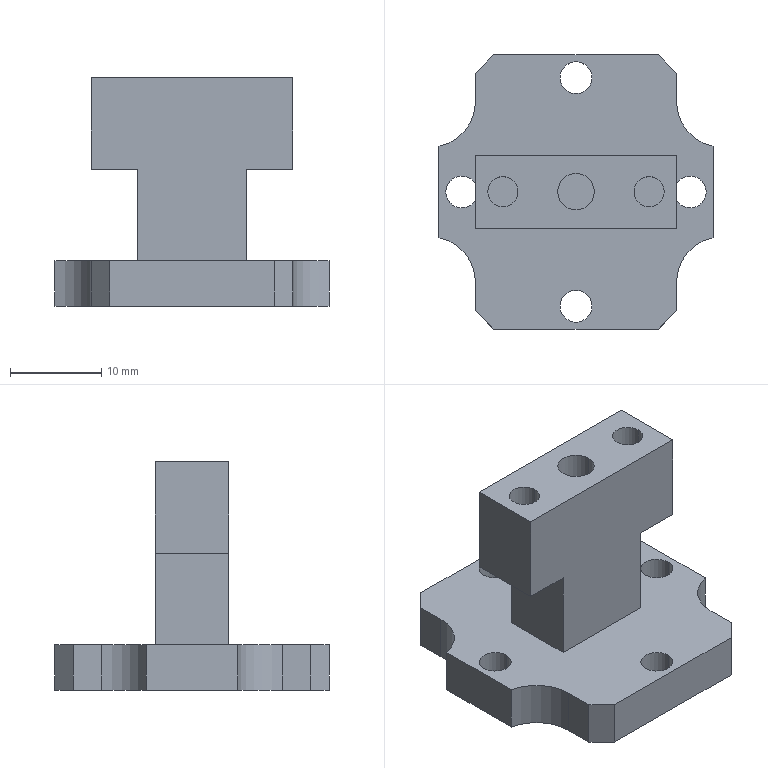Part | STEP file | 08-20 rotary support seat | 1 solid | 42 faces | box 30 x 30 x 25 mm | volume 6052 mm3 | plane 24 | cylinder 18 | commonest cylinder face diameters 3.5 x8 3.3 x4 10 x4 4 x2
STEP:
#1=CARTESIAN_POINT('',(10.75,0.,0.));
#2=VERTEX_POINT('',#1);
#3=CARTESIAN_POINT('',(14.25,0.,0.));
#4=VERTEX_POINT('',#3);
#5=CARTESIAN_POINT('',(12.5,0.,0.));
#6=DIRECTION('',(0.,0.,1.));
#7=DIRECTION('',(1.,0.,0.));
#8=AXIS2_PLACEMENT_3D('',#5,#6,#7);
#9=CIRCLE('',#8,1.75);
#10=EDGE_CURVE('',#2,#4,#9,.T.);
#11=ORIENTED_EDGE('',*,*,#10,.F.);
#12=CARTESIAN_POINT('',(10.75,0.,5.));
#13=VERTEX_POINT('',#12);
#14=CARTESIAN_POINT('',(10.75,0.,-5.));
#15=DIRECTION('',(0.,0.,1.));
#16=VECTOR('',#15,1000.);
#17=LINE('',#14,#16);
#18=EDGE_CURVE('',#2,#13,#17,.T.);
#19=ORIENTED_EDGE('',*,*,#18,.T.);
#20=CARTESIAN_POINT('',(14.25,0.,5.));
#21=VERTEX_POINT('',#20);
#22=CARTESIAN_POINT('',(12.5,0.,5.));
#23=DIRECTION('',(0.,0.,1.));
#24=DIRECTION('',(0.,1.,0.));
#25=AXIS2_PLACEMENT_3D('',#22,#23,#24);
#26=CIRCLE('',#25,1.75);
#27=EDGE_CURVE('',#13,#21,#26,.T.);
#28=ORIENTED_EDGE('',*,*,#27,.T.);
#29=CARTESIAN_POINT('',(14.25,0.,-5.));
#30=DIRECTION('',(0.,0.,1.));
#31=VECTOR('',#30,1000.);
#32=LINE('',#29,#31);
#33=EDGE_CURVE('',#4,#21,#32,.T.);
#34=ORIENTED_EDGE('',*,*,#33,.F.);
#35=EDGE_LOOP('',(#11,#19,#28,#34));
#36=FACE_OUTER_BOUND('',#35,.T.);
#37=CARTESIAN_POINT('',(12.5,0.,-5.));
#38=DIRECTION('',(0.,0.,1.));
#39=DIRECTION('',(1.,0.,0.));
#40=AXIS2_PLACEMENT_3D('',#37,#38,#39);
#41=CYLINDRICAL_SURFACE('',#40,1.75);
#42=ADVANCED_FACE('',(#36),#41,.F.);
#43=CARTESIAN_POINT('',(-14.25,0.,0.));
#44=VERTEX_POINT('',#43);
#45=CARTESIAN_POINT('',(-10.75,0.,0.));
#46=VERTEX_POINT('',#45);
#47=CARTESIAN_POINT('',(-12.5,0.,0.));
#48=DIRECTION('',(0.,0.,1.));
#49=DIRECTION('',(1.,0.,0.));
#50=AXIS2_PLACEMENT_3D('',#47,#48,#49);
#51=CIRCLE('',#50,1.75);
#52=EDGE_CURVE('',#44,#46,#51,.T.);
#53=ORIENTED_EDGE('',*,*,#52,.F.);
#54=CARTESIAN_POINT('',(-14.25,0.,5.));
#55=VERTEX_POINT('',#54);
#56=CARTESIAN_POINT('',(-14.25,0.,-5.));
#57=DIRECTION('',(0.,0.,1.));
#58=VECTOR('',#57,1000.);
#59=LINE('',#56,#58);
#60=EDGE_CURVE('',#44,#55,#59,.T.);
#61=ORIENTED_EDGE('',*,*,#60,.T.);
#62=CARTESIAN_POINT('',(-10.75,0.,5.));
#63=VERTEX_POINT('',#62);
#64=CARTESIAN_POINT('',(-12.5,0.,5.));
#65=DIRECTION('',(0.,0.,1.));
#66=DIRECTION('',(0.,1.,0.));
#67=AXIS2_PLACEMENT_3D('',#64,#65,#66);
#68=CIRCLE('',#67,1.75);
#69=EDGE_CURVE('',#55,#63,#68,.T.);
#70=ORIENTED_EDGE('',*,*,#69,.T.);
#71=CARTESIAN_POINT('',(-10.75,0.,-5.));
#72=DIRECTION('',(0.,0.,1.));
#73=VECTOR('',#72,1000.);
#74=LINE('',#71,#73);
#75=EDGE_CURVE('',#46,#63,#74,.T.);
#76=ORIENTED_EDGE('',*,*,#75,.F.);
#77=EDGE_LOOP('',(#53,#61,#70,#76));
#78=FACE_OUTER_BOUND('',#77,.T.);
#79=CARTESIAN_POINT('',(-12.5,0.,-5.));
#80=DIRECTION('',(0.,0.,1.));
#81=DIRECTION('',(1.,0.,0.));
#82=AXIS2_PLACEMENT_3D('',#79,#80,#81);
#83=CYLINDRICAL_SURFACE('',#82,1.75);
#84=ADVANCED_FACE('',(#78),#83,.F.);
#85=CARTESIAN_POINT('',(-1.75,-12.5,0.));
#86=VERTEX_POINT('',#85);
#87=CARTESIAN_POINT('',(1.75,-12.5,0.));
#88=VERTEX_POINT('',#87);
#89=CARTESIAN_POINT('',(0.,-12.5,0.));
#90=DIRECTION('',(0.,0.,1.));
#91=DIRECTION('',(1.,0.,0.));
#92=AXIS2_PLACEMENT_3D('',#89,#90,#91);
#93=CIRCLE('',#92,1.75);
#94=EDGE_CURVE('',#86,#88,#93,.T.);
#95=ORIENTED_EDGE('',*,*,#94,.F.);
#96=CARTESIAN_POINT('',(-1.75,-12.5,5.));
#97=VERTEX_POINT('',#96);
#98=CARTESIAN_POINT('',(-1.75,-12.5,-5.));
#99=DIRECTION('',(0.,0.,1.));
#100=VECTOR('',#99,1000.);
#101=LINE('',#98,#100);
#102=EDGE_CURVE('',#86,#97,#101,.T.);
#103=ORIENTED_EDGE('',*,*,#102,.T.);
#104=CARTESIAN_POINT('',(1.75,-12.5,5.));
#105=VERTEX_POINT('',#104);
#106=CARTESIAN_POINT('',(0.,-12.5,5.));
#107=DIRECTION('',(0.,0.,1.));
#108=DIRECTION('',(1.,0.,0.));
#109=AXIS2_PLACEMENT_3D('',#106,#107,#108);
#110=CIRCLE('',#109,1.75);
#111=EDGE_CURVE('',#97,#105,#110,.T.);
#112=ORIENTED_EDGE('',*,*,#111,.T.);
#113=CARTESIAN_POINT('',(1.75,-12.5,-5.));
#114=DIRECTION('',(0.,0.,1.));
#115=VECTOR('',#114,1000.);
#116=LINE('',#113,#115);
#117=EDGE_CURVE('',#88,#105,#116,.T.);
#118=ORIENTED_EDGE('',*,*,#117,.F.);
#119=EDGE_LOOP('',(#95,#103,#112,#118));
#120=FACE_OUTER_BOUND('',#119,.T.);
#121=CARTESIAN_POINT('',(0.,-12.5,-5.));
#122=DIRECTION('',(0.,0.,1.));
#123=DIRECTION('',(1.,0.,0.));
#124=AXIS2_PLACEMENT_3D('',#121,#122,#123);
#125=CYLINDRICAL_SURFACE('',#124,1.75);
#126=ADVANCED_FACE('',(#120),#125,.F.);
#127=CARTESIAN_POINT('',(-1.75,12.5,0.));
#128=VERTEX_POINT('',#127);
#129=CARTESIAN_POINT('',(1.75,12.5,0.));
#130=VERTEX_POINT('',#129);
#131=CARTESIAN_POINT('',(0.,12.5,0.));
#132=DIRECTION('',(0.,0.,1.));
#133=DIRECTION('',(1.,0.,0.));
#134=AXIS2_PLACEMENT_3D('',#131,#132,#133);
#135=CIRCLE('',#134,1.75);
#136=EDGE_CURVE('',#128,#130,#135,.T.);
#137=ORIENTED_EDGE('',*,*,#136,.F.);
#138=CARTESIAN_POINT('',(-1.75,12.5,5.));
#139=VERTEX_POINT('',#138);
#140=CARTESIAN_POINT('',(-1.75,12.5,-5.));
#141=DIRECTION('',(0.,0.,1.));
#142=VECTOR('',#141,1000.);
#143=LINE('',#140,#142);
#144=EDGE_CURVE('',#128,#139,#143,.T.);
#145=ORIENTED_EDGE('',*,*,#144,.T.);
#146=CARTESIAN_POINT('',(1.75,12.5,5.));
#147=VERTEX_POINT('',#146);
#148=CARTESIAN_POINT('',(0.,12.5,5.));
#149=DIRECTION('',(0.,0.,1.));
#150=DIRECTION('',(1.,0.,0.));
#151=AXIS2_PLACEMENT_3D('',#148,#149,#150);
#152=CIRCLE('',#151,1.75);
#153=EDGE_CURVE('',#139,#147,#152,.T.);
#154=ORIENTED_EDGE('',*,*,#153,.T.);
#155=CARTESIAN_POINT('',(1.75,12.5,-5.));
#156=DIRECTION('',(0.,0.,1.));
#157=VECTOR('',#156,1000.);
#158=LINE('',#155,#157);
#159=EDGE_CURVE('',#130,#147,#158,.T.);
#160=ORIENTED_EDGE('',*,*,#159,.F.);
#161=EDGE_LOOP('',(#137,#145,#154,#160));
#162=FACE_OUTER_BOUND('',#161,.T.);
#163=CARTESIAN_POINT('',(0.,12.5,-5.));
#164=DIRECTION('',(0.,0.,1.));
#165=DIRECTION('',(1.,0.,0.));
#166=AXIS2_PLACEMENT_3D('',#163,#164,#165);
#167=CYLINDRICAL_SURFACE('',#166,1.75);
#168=ADVANCED_FACE('',(#162),#167,.F.);
#169=CARTESIAN_POINT('',(-6.35,0.,15.));
#170=VERTEX_POINT('',#169);
#171=CARTESIAN_POINT('',(-9.65,0.,15.));
#172=VERTEX_POINT('',#171);
#173=CARTESIAN_POINT('',(-8.,0.,15.));
#174=DIRECTION('',(0.,0.,-1.));
#175=DIRECTION('',(1.,0.,0.));
#176=AXIS2_PLACEMENT_3D('',#173,#174,#175);
#177=CIRCLE('',#176,1.65);
#178=EDGE_CURVE('',#170,#172,#177,.T.);
#179=ORIENTED_EDGE('',*,*,#178,.T.);
#180=CARTESIAN_POINT('',(-9.65,0.,25.));
#181=VERTEX_POINT('',#180);
#182=CARTESIAN_POINT('',(-9.65,0.,25.));
#183=DIRECTION('',(0.,0.,1.));
#184=VECTOR('',#183,1000.);
#185=LINE('',#182,#184);
#186=EDGE_CURVE('',#172,#181,#185,.T.);
#187=ORIENTED_EDGE('',*,*,#186,.T.);
#188=CARTESIAN_POINT('',(-6.35,0.,25.));
#189=VERTEX_POINT('',#188);
#190=CARTESIAN_POINT('',(-8.,0.,25.));
#191=DIRECTION('',(0.,0.,1.));
#192=DIRECTION('',(1.,0.,0.));
#193=AXIS2_PLACEMENT_3D('',#190,#191,#192);
#194=CIRCLE('',#193,1.65);
#195=EDGE_CURVE('',#181,#189,#194,.T.);
#196=ORIENTED_EDGE('',*,*,#195,.T.);
#197=CARTESIAN_POINT('',(-6.35,0.,25.));
#198=DIRECTION('',(0.,0.,1.));
#199=VECTOR('',#198,1000.);
#200=LINE('',#197,#199);
#201=EDGE_CURVE('',#170,#189,#200,.T.);
#202=ORIENTED_EDGE('',*,*,#201,.F.);
#203=EDGE_LOOP('',(#179,#187,#196,#202));
#204=FACE_OUTER_BOUND('',#203,.T.);
#205=CARTESIAN_POINT('',(-8.,0.,25.));
#206=DIRECTION('',(0.,0.,1.));
#207=DIRECTION('',(1.,0.,0.));
#208=AXIS2_PLACEMENT_3D('',#205,#206,#207);
#209=CYLINDRICAL_SURFACE('',#208,1.65);
#210=ADVANCED_FACE('',(#204),#209,.F.);
#211=CARTESIAN_POINT('',(9.65,0.,15.));
#212=VERTEX_POINT('',#211);
#213=CARTESIAN_POINT('',(6.35,0.,15.));
#214=VERTEX_POINT('',#213);
#215=CARTESIAN_POINT('',(8.,0.,15.));
#216=DIRECTION('',(0.,0.,-1.));
#217=DIRECTION('',(1.,0.,0.));
#218=AXIS2_PLACEMENT_3D('',#215,#216,#217);
#219=CIRCLE('',#218,1.65);
#220=EDGE_CURVE('',#212,#214,#219,.T.);
#221=ORIENTED_EDGE('',*,*,#220,.T.);
#222=CARTESIAN_POINT('',(6.35,0.,25.));
#223=VERTEX_POINT('',#222);
#224=CARTESIAN_POINT('',(6.35,0.,25.));
#225=DIRECTION('',(0.,0.,1.));
#226=VECTOR('',#225,1000.);
#227=LINE('',#224,#226);
#228=EDGE_CURVE('',#214,#223,#227,.T.);
#229=ORIENTED_EDGE('',*,*,#228,.T.);
#230=CARTESIAN_POINT('',(9.65,0.,25.));
#231=VERTEX_POINT('',#230);
#232=CARTESIAN_POINT('',(8.,0.,25.));
#233=DIRECTION('',(0.,0.,1.));
#234=DIRECTION('',(1.,0.,0.));
#235=AXIS2_PLACEMENT_3D('',#232,#233,#234);
#236=CIRCLE('',#235,1.65);
#237=EDGE_CURVE('',#223,#231,#236,.T.);
#238=ORIENTED_EDGE('',*,*,#237,.T.);
#239=CARTESIAN_POINT('',(9.65,0.,25.));
#240=DIRECTION('',(0.,0.,1.));
#241=VECTOR('',#240,1000.);
#242=LINE('',#239,#241);
#243=EDGE_CURVE('',#212,#231,#242,.T.);
#244=ORIENTED_EDGE('',*,*,#243,.F.);
#245=EDGE_LOOP('',(#221,#229,#238,#244));
#246=FACE_OUTER_BOUND('',#245,.T.);
#247=CARTESIAN_POINT('',(8.,0.,25.));
#248=DIRECTION('',(0.,0.,1.));
#249=DIRECTION('',(1.,0.,0.));
#250=AXIS2_PLACEMENT_3D('',#247,#248,#249);
#251=CYLINDRICAL_SURFACE('',#250,1.65);
#252=ADVANCED_FACE('',(#246),#251,.F.);
#253=CARTESIAN_POINT('',(-2.,0.,20.));
#254=VERTEX_POINT('',#253);
#255=CARTESIAN_POINT('',(2.,0.,20.));
#256=VERTEX_POINT('',#255);
#257=CARTESIAN_POINT('',(0.,0.,20.));
#258=DIRECTION('',(0.,0.,1.));
#259=DIRECTION('',(1.,0.,0.));
#260=AXIS2_PLACEMENT_3D('',#257,#258,#259);
#261=CIRCLE('',#260,2.);
#262=EDGE_CURVE('',#254,#256,#261,.T.);
#263=ORIENTED_EDGE('',*,*,#262,.F.);
#264=CARTESIAN_POINT('',(-2.,0.,25.));
#265=VERTEX_POINT('',#264);
#266=CARTESIAN_POINT('',(-2.,0.,20.));
#267=DIRECTION('',(0.,0.,1.));
#268=VECTOR('',#267,1000.);
#269=LINE('',#266,#268);
#270=EDGE_CURVE('',#254,#265,#269,.T.);
#271=ORIENTED_EDGE('',*,*,#270,.T.);
#272=CARTESIAN_POINT('',(2.,0.,25.));
#273=VERTEX_POINT('',#272);
#274=CARTESIAN_POINT('',(0.,0.,25.));
#275=DIRECTION('',(0.,0.,1.));
#276=DIRECTION('',(1.,0.,0.));
#277=AXIS2_PLACEMENT_3D('',#274,#275,#276);
#278=CIRCLE('',#277,2.);
#279=EDGE_CURVE('',#265,#273,#278,.T.);
#280=ORIENTED_EDGE('',*,*,#279,.T.);
#281=CARTESIAN_POINT('',(2.,0.,20.));
#282=DIRECTION('',(0.,0.,1.));
#283=VECTOR('',#282,1000.);
#284=LINE('',#281,#283);
#285=EDGE_CURVE('',#256,#273,#284,.T.);
#286=ORIENTED_EDGE('',*,*,#285,.F.);
#287=EDGE_LOOP('',(#263,#271,#280,#286));
#288=FACE_OUTER_BOUND('',#287,.T.);
#289=CARTESIAN_POINT('',(0.,0.,20.));
#290=DIRECTION('',(0.,0.,1.));
#291=DIRECTION('',(1.,0.,0.));
#292=AXIS2_PLACEMENT_3D('',#289,#290,#291);
#293=CYLINDRICAL_SURFACE('',#292,2.);
#294=ADVANCED_FACE('',(#288),#293,.F.);
#295=CARTESIAN_POINT('',(11.,9.899,5.));
#296=VERTEX_POINT('',#295);
#297=CARTESIAN_POINT('',(11.,13.,5.));
#298=VERTEX_POINT('',#297);
#299=CARTESIAN_POINT('',(11.,15.,5.));
#300=DIRECTION('',(0.,1.,0.));
#301=VECTOR('',#300,1000.);
#302=LINE('',#299,#301);
#303=EDGE_CURVE('',#296,#298,#302,.T.);
#304=ORIENTED_EDGE('',*,*,#303,.F.);
#305=CARTESIAN_POINT('',(11.,9.899,0.));
#306=VERTEX_POINT('',#305);
#307=CARTESIAN_POINT('',(11.,9.899,5.));
#308=DIRECTION('',(0.,0.,-1.));
#309=VECTOR('',#308,1000.);
#310=LINE('',#307,#309);
#311=EDGE_CURVE('',#296,#306,#310,.T.);
#312=ORIENTED_EDGE('',*,*,#311,.T.);
#313=CARTESIAN_POINT('',(11.,13.,0.));
#314=VERTEX_POINT('',#313);
#315=CARTESIAN_POINT('',(11.,15.,0.));
#316=DIRECTION('',(0.,1.,0.));
#317=VECTOR('',#316,1000.);
#318=LINE('',#315,#317);
#319=EDGE_CURVE('',#306,#314,#318,.T.);
#320=ORIENTED_EDGE('',*,*,#319,.T.);
#321=CARTESIAN_POINT('',(11.,13.,5.));
#322=DIRECTION('',(0.,0.,1.));
#323=VECTOR('',#322,1000.);
#324=LINE('',#321,#323);
#325=EDGE_CURVE('',#314,#298,#324,.T.);
#326=ORIENTED_EDGE('',*,*,#325,.T.);
#327=EDGE_LOOP('',(#304,#312,#320,#326));
#328=FACE_OUTER_BOUND('',#327,.T.);
#329=CARTESIAN_POINT('',(11.,15.,5.));
#330=DIRECTION('',(-1.,0.,0.));
#331=DIRECTION('',(0.,-1.,0.));
#332=AXIS2_PLACEMENT_3D('',#329,#330,#331);
#333=PLANE('',#332);
#334=ADVANCED_FACE('',(#328),#333,.F.);
#335=CARTESIAN_POINT('',(11.,-4.,25.));
#336=VERTEX_POINT('',#335);
#337=CARTESIAN_POINT('',(11.,-4.,15.));
#338=VERTEX_POINT('',#337);
#339=CARTESIAN_POINT('',(11.,-4.,25.));
#340=DIRECTION('',(0.,0.,-1.));
#341=VECTOR('',#340,1000.);
#342=LINE('',#339,#341);
#343=EDGE_CURVE('',#336,#338,#342,.T.);
#344=ORIENTED_EDGE('',*,*,#343,.T.);
#345=CARTESIAN_POINT('',(11.,4.,15.));
#346=VERTEX_POINT('',#345);
#347=CARTESIAN_POINT('',(11.,-6.,15.));
#348=DIRECTION('',(0.,1.,0.));
#349=VECTOR('',#348,1000.);
#350=LINE('',#347,#349);
#351=EDGE_CURVE('',#338,#346,#350,.T.);
#352=ORIENTED_EDGE('',*,*,#351,.T.);
#353=CARTESIAN_POINT('',(11.,4.,25.));
#354=VERTEX_POINT('',#353);
#355=CARTESIAN_POINT('',(11.,4.,25.));
#356=DIRECTION('',(0.,0.,-1.));
#357=VECTOR('',#356,1000.);
#358=LINE('',#355,#357);
#359=EDGE_CURVE('',#354,#346,#358,.T.);
#360=ORIENTED_EDGE('',*,*,#359,.F.);
#361=CARTESIAN_POINT('',(11.,4.,25.));
#362=DIRECTION('',(0.,1.,0.));
#363=VECTOR('',#362,1000.);
#364=LINE('',#361,#363);
#365=EDGE_CURVE('',#336,#354,#364,.T.);
#366=ORIENTED_EDGE('',*,*,#365,.F.);
#367=EDGE_LOOP('',(#344,#352,#360,#366));
#368=FACE_OUTER_BOUND('',#367,.T.);
#369=CARTESIAN_POINT('',(11.,15.,5.));
#370=DIRECTION('',(-1.,0.,0.));
#371=DIRECTION('',(0.,-1.,0.));
#372=AXIS2_PLACEMENT_3D('',#369,#370,#371);
#373=PLANE('',#372);
#374=ADVANCED_FACE('',(#368),#373,.F.);
#375=CARTESIAN_POINT('',(-11.,13.,0.));
#376=VERTEX_POINT('',#375);
#377=CARTESIAN_POINT('',(-11.,9.899,0.));
#378=VERTEX_POINT('',#377);
#379=CARTESIAN_POINT('',(-11.,15.,0.));
#380=DIRECTION('',(0.,-1.,0.));
#381=VECTOR('',#380,1000.);
#382=LINE('',#379,#381);
#383=EDGE_CURVE('',#376,#378,#382,.T.);
#384=ORIENTED_EDGE('',*,*,#383,.T.);
#385=CARTESIAN_POINT('',(-11.,9.899,5.));
#386=VERTEX_POINT('',#385);
#387=CARTESIAN_POINT('',(-11.,9.899,5.));
#388=DIRECTION('',(0.,0.,1.));
#389=VECTOR('',#388,1000.);
#390=LINE('',#387,#389);
#391=EDGE_CURVE('',#378,#386,#390,.T.);
#392=ORIENTED_EDGE('',*,*,#391,.T.);
#393=CARTESIAN_POINT('',(-11.,13.,5.));
#394=VERTEX_POINT('',#393);
#395=CARTESIAN_POINT('',(-11.,15.,5.));
#396=DIRECTION('',(0.,-1.,0.));
#397=VECTOR('',#396,1000.);
#398=LINE('',#395,#397);
#399=EDGE_CURVE('',#394,#386,#398,.T.);
#400=ORIENTED_EDGE('',*,*,#399,.F.);
#401=CARTESIAN_POINT('',(-11.,13.,5.));
#402=DIRECTION('',(0.,0.,-1.));
#403=VECTOR('',#402,1000.);
#404=LINE('',#401,#403);
#405=EDGE_CURVE('',#394,#376,#404,.T.);
#406=ORIENTED_EDGE('',*,*,#405,.T.);
#407=EDGE_LOOP('',(#384,#392,#400,#406));
#408=FACE_OUTER_BOUND('',#407,.T.);
#409=CARTESIAN_POINT('',(-11.,15.,5.));
#410=DIRECTION('',(1.,0.,0.));
#411=DIRECTION('',(0.,1.,0.));
#412=AXIS2_PLACEMENT_3D('',#409,#410,#411);
#413=PLANE('',#412);
#414=ADVANCED_FACE('',(#408),#413,.F.);
#415=CARTESIAN_POINT('',(-11.,4.,25.));
#416=VERTEX_POINT('',#415);
#417=CARTESIAN_POINT('',(-11.,4.,15.));
#418=VERTEX_POINT('',#417);
#419=CARTESIAN_POINT('',(-11.,4.,25.));
#420=DIRECTION('',(0.,0.,-1.));
#421=VECTOR('',#420,1000.);
#422=LINE('',#419,#421);
#423=EDGE_CURVE('',#416,#418,#422,.T.);
#424=ORIENTED_EDGE('',*,*,#423,.T.);
#425=CARTESIAN_POINT('',(-11.,-4.,15.));
#426=VERTEX_POINT('',#425);
#427=CARTESIAN_POINT('',(-11.,-6.,15.));
#428=DIRECTION('',(0.,1.,0.));
#429=VECTOR('',#428,1000.);
#430=LINE('',#427,#429);
#431=EDGE_CURVE('',#426,#418,#430,.T.);
#432=ORIENTED_EDGE('',*,*,#431,.F.);
#433=CARTESIAN_POINT('',(-11.,-4.,25.));
#434=VERTEX_POINT('',#433);
#435=CARTESIAN_POINT('',(-11.,-4.,25.));
#436=DIRECTION('',(0.,0.,-1.));
#437=VECTOR('',#436,1000.);
#438=LINE('',#435,#437);
#439=EDGE_CURVE('',#434,#426,#438,.T.);
#440=ORIENTED_EDGE('',*,*,#439,.F.);
#441=CARTESIAN_POINT('',(-11.,4.,25.));
#442=DIRECTION('',(0.,-1.,0.));
#443=VECTOR('',#442,1000.);
#444=LINE('',#441,#443);
#445=EDGE_CURVE('',#416,#434,#444,.T.);
#446=ORIENTED_EDGE('',*,*,#445,.F.);
#447=EDGE_LOOP('',(#424,#432,#440,#446));
#448=FACE_OUTER_BOUND('',#447,.T.);
#449=CARTESIAN_POINT('',(-11.,15.,5.));
#450=DIRECTION('',(1.,0.,0.));
#451=DIRECTION('',(0.,1.,0.));
#452=AXIS2_PLACEMENT_3D('',#449,#450,#451);
#453=PLANE('',#452);
#454=ADVANCED_FACE('',(#448),#453,.F.);
#455=CARTESIAN_POINT('',(11.,-13.,0.));
#456=VERTEX_POINT('',#455);
#457=CARTESIAN_POINT('',(11.,-9.899,0.));
#458=VERTEX_POINT('',#457);
#459=CARTESIAN_POINT('',(11.,15.,0.));
#460=DIRECTION('',(0.,1.,0.));
#461=VECTOR('',#460,1000.);
#462=LINE('',#459,#461);
#463=EDGE_CURVE('',#456,#458,#462,.T.);
#464=ORIENTED_EDGE('',*,*,#463,.T.);
#465=CARTESIAN_POINT('',(11.,-9.899,5.));
#466=VERTEX_POINT('',#465);
#467=CARTESIAN_POINT('',(11.,-9.899,5.));
#468=DIRECTION('',(0.,0.,1.));
#469=VECTOR('',#468,1000.);
#470=LINE('',#467,#469);
#471=EDGE_CURVE('',#458,#466,#470,.T.);
#472=ORIENTED_EDGE('',*,*,#471,.T.);
#473=CARTESIAN_POINT('',(11.,-13.,5.));
#474=VERTEX_POINT('',#473);
#475=CARTESIAN_POINT('',(11.,15.,5.));
#476=DIRECTION('',(0.,1.,0.));
#477=VECTOR('',#476,1000.);
#478=LINE('',#475,#477);
#479=EDGE_CURVE('',#474,#466,#478,.T.);
#480=ORIENTED_EDGE('',*,*,#479,.F.);
#481=CARTESIAN_POINT('',(11.,-13.,5.));
#482=DIRECTION('',(0.,0.,-1.));
#483=VECTOR('',#482,1000.);
#484=LINE('',#481,#483);
#485=EDGE_CURVE('',#474,#456,#484,.T.);
#486=ORIENTED_EDGE('',*,*,#485,.T.);
#487=EDGE_LOOP('',(#464,#472,#480,#486));
#488=FACE_OUTER_BOUND('',#487,.T.);
#489=CARTESIAN_POINT('',(11.,15.,5.));
#490=DIRECTION('',(-1.,0.,0.));
#491=DIRECTION('',(0.,-1.,0.));
#492=AXIS2_PLACEMENT_3D('',#489,#490,#491);
#493=PLANE('',#492);
#494=ADVANCED_FACE('',(#488),#493,.F.);
#495=CARTESIAN_POINT('',(9.,15.,5.));
#496=VERTEX_POINT('',#495);
#497=CARTESIAN_POINT('',(-9.,15.,5.));
#498=VERTEX_POINT('',#497);
#499=CARTESIAN_POINT('',(-11.,15.,5.));
#500=DIRECTION('',(-1.,0.,0.));
#501=VECTOR('',#500,1000.);
#502=LINE('',#499,#501);
#503=EDGE_CURVE('',#496,#498,#502,.T.);
#504=ORIENTED_EDGE('',*,*,#503,.F.);
#505=CARTESIAN_POINT('',(9.,15.,0.));
#506=VERTEX_POINT('',#505);
#507=CARTESIAN_POINT('',(9.,15.,5.));
#508=DIRECTION('',(0.,0.,-1.));
#509=VECTOR('',#508,1000.);
#510=LINE('',#507,#509);
#511=EDGE_CURVE('',#496,#506,#510,.T.);
#512=ORIENTED_EDGE('',*,*,#511,.T.);
#513=CARTESIAN_POINT('',(-9.,15.,0.));
#514=VERTEX_POINT('',#513);
#515=CARTESIAN_POINT('',(-11.,15.,0.));
#516=DIRECTION('',(-1.,0.,0.));
#517=VECTOR('',#516,1000.);
#518=LINE('',#515,#517);
#519=EDGE_CURVE('',#506,#514,#518,.T.);
#520=ORIENTED_EDGE('',*,*,#519,.T.);
#521=CARTESIAN_POINT('',(-9.,15.,5.));
#522=DIRECTION('',(0.,0.,1.));
#523=VECTOR('',#522,1000.);
#524=LINE('',#521,#523);
#525=EDGE_CURVE('',#514,#498,#524,.T.);
#526=ORIENTED_EDGE('',*,*,#525,.T.);
#527=EDGE_LOOP('',(#504,#512,#520,#526));
#528=FACE_OUTER_BOUND('',#527,.T.);
#529=CARTESIAN_POINT('',(-11.,15.,5.));
#530=DIRECTION('',(0.,-1.,0.));
#531=DIRECTION('',(0.,0.,-1.));
#532=AXIS2_PLACEMENT_3D('',#529,#530,#531);
#533=PLANE('',#532);
#534=ADVANCED_FACE('',(#528),#533,.F.);
#535=CARTESIAN_POINT('',(-11.,-9.899,5.));
#536=VERTEX_POINT('',#535);
#537=CARTESIAN_POINT('',(-11.,-13.,5.));
#538=VERTEX_POINT('',#537);
#539=CARTESIAN_POINT('',(-11.,15.,5.));
#540=DIRECTION('',(0.,-1.,0.));
#541=VECTOR('',#540,1000.);
#542=LINE('',#539,#541);
#543=EDGE_CURVE('',#536,#538,#542,.T.);
#544=ORIENTED_EDGE('',*,*,#543,.F.);
#545=CARTESIAN_POINT('',(-11.,-9.899,0.));
#546=VERTEX_POINT('',#545);
#547=CARTESIAN_POINT('',(-11.,-9.899,5.));
#548=DIRECTION('',(0.,0.,-1.));
#549=VECTOR('',#548,1000.);
#550=LINE('',#547,#549);
#551=EDGE_CURVE('',#536,#546,#550,.T.);
#552=ORIENTED_EDGE('',*,*,#551,.T.);
#553=CARTESIAN_POINT('',(-11.,-13.,0.));
#554=VERTEX_POINT('',#553);
#555=CARTESIAN_POINT('',(-11.,15.,0.));
#556=DIRECTION('',(0.,-1.,0.));
#557=VECTOR('',#556,1000.);
#558=LINE('',#555,#557);
#559=EDGE_CURVE('',#546,#554,#558,.T.);
#560=ORIENTED_EDGE('',*,*,#559,.T.);
#561=CARTESIAN_POINT('',(-11.,-13.,5.));
#562=DIRECTION('',(0.,0.,1.));
#563=VECTOR('',#562,1000.);
#564=LINE('',#561,#563);
#565=EDGE_CURVE('',#554,#538,#564,.T.);
#566=ORIENTED_EDGE('',*,*,#565,.T.);
#567=EDGE_LOOP('',(#544,#552,#560,#566));
#568=FACE_OUTER_BOUND('',#567,.T.);
#569=CARTESIAN_POINT('',(-11.,15.,5.));
#570=DIRECTION('',(1.,0.,0.));
#571=DIRECTION('',(0.,1.,0.));
#572=AXIS2_PLACEMENT_3D('',#569,#570,#571);
#573=PLANE('',#572);
#574=ADVANCED_FACE('',(#568),#573,.F.);
#575=CARTESIAN_POINT('',(-9.,-15.,5.));
#576=VERTEX_POINT('',#575);
#577=CARTESIAN_POINT('',(9.,-15.,5.));
#578=VERTEX_POINT('',#577);
#579=CARTESIAN_POINT('',(-11.,-15.,5.));
#580=DIRECTION('',(1.,0.,0.));
#581=VECTOR('',#580,1000.);
#582=LINE('',#579,#581);
#583=EDGE_CURVE('',#576,#578,#582,.T.);
#584=ORIENTED_EDGE('',*,*,#583,.F.);
#585=CARTESIAN_POINT('',(-9.,-15.,0.));
#586=VERTEX_POINT('',#585);
#587=CARTESIAN_POINT('',(-9.,-15.,5.));
#588=DIRECTION('',(0.,0.,-1.));
#589=VECTOR('',#588,1000.);
#590=LINE('',#587,#589);
#591=EDGE_CURVE('',#576,#586,#590,.T.);
#592=ORIENTED_EDGE('',*,*,#591,.T.);
#593=CARTESIAN_POINT('',(9.,-15.,0.));
#594=VERTEX_POINT('',#593);
#595=CARTESIAN_POINT('',(-11.,-15.,0.));
#596=DIRECTION('',(1.,0.,0.));
#597=VECTOR('',#596,1000.);
#598=LINE('',#595,#597);
#599=EDGE_CURVE('',#586,#594,#598,.T.);
#600=ORIENTED_EDGE('',*,*,#599,.T.);
#601=CARTESIAN_POINT('',(9.,-15.,5.));
#602=DIRECTION('',(0.,0.,1.));
#603=VECTOR('',#602,1000.);
#604=LINE('',#601,#603);
#605=EDGE_CURVE('',#594,#578,#604,.T.);
#606=ORIENTED_EDGE('',*,*,#605,.T.);
#607=EDGE_LOOP('',(#584,#592,#600,#606));
#608=FACE_OUTER_BOUND('',#607,.T.);
#609=CARTESIAN_POINT('',(-11.,-15.,5.));
#610=DIRECTION('',(0.,1.,0.));
#611=DIRECTION('',(0.,0.,1.));
#612=AXIS2_PLACEMENT_3D('',#609,#610,#611);
#613=PLANE('',#612);
#614=ADVANCED_FACE('',(#608),#613,.F.);
#615=CARTESIAN_POINT('',(12.5,0.,5.));
#616=DIRECTION('',(0.,0.,1.));
#617=DIRECTION('',(0.,1.,0.));
#618=AXIS2_PLACEMENT_3D('',#615,#616,#617);
#619=CIRCLE('',#618,1.75);
#620=EDGE_CURVE('',#21,#13,#619,.T.);
#621=ORIENTED_EDGE('',*,*,#620,.F.);
#622=ORIENTED_EDGE('',*,*,#27,.F.);
#623=EDGE_LOOP('',(#621,#622));
#624=FACE_BOUND('',#623,.T.);
#625=CARTESIAN_POINT('',(6.,-4.,5.));
#626=VERTEX_POINT('',#625);
#627=CARTESIAN_POINT('',(6.,4.,5.));
#628=VERTEX_POINT('',#627);
#629=CARTESIAN_POINT('',(6.,-6.,5.));
#630=DIRECTION('',(0.,1.,0.));
#631=VECTOR('',#630,1000.);
#632=LINE('',#629,#631);
#633=EDGE_CURVE('',#626,#628,#632,.T.);
#634=ORIENTED_EDGE('',*,*,#633,.F.);
#635=CARTESIAN_POINT('',(-6.,-4.,5.));
#636=VERTEX_POINT('',#635);
#637=CARTESIAN_POINT('',(-11.,-4.,5.));
#638=DIRECTION('',(1.,0.,0.));
#639=VECTOR('',#638,1000.);
#640=LINE('',#637,#639);
#641=EDGE_CURVE('',#636,#626,#640,.T.);
#642=ORIENTED_EDGE('',*,*,#641,.F.);
#643=CARTESIAN_POINT('',(-6.,4.,5.));
#644=VERTEX_POINT('',#643);
#645=CARTESIAN_POINT('',(-6.,-6.,5.));
#646=DIRECTION('',(0.,1.,0.));
#647=VECTOR('',#646,1000.);
#648=LINE('',#645,#647);
#649=EDGE_CURVE('',#636,#644,#648,.T.);
#650=ORIENTED_EDGE('',*,*,#649,.T.);
#651=CARTESIAN_POINT('',(-11.,4.,5.));
#652=DIRECTION('',(-1.,0.,0.));
#653=VECTOR('',#652,1000.);
#654=LINE('',#651,#653);
#655=EDGE_CURVE('',#628,#644,#654,.T.);
#656=ORIENTED_EDGE('',*,*,#655,.F.);
#657=EDGE_LOOP('',(#634,#642,#650,#656));
#658=FACE_BOUND('',#657,.T.);
#659=CARTESIAN_POINT('',(-12.5,0.,5.));
#660=DIRECTION('',(0.,0.,1.));
#661=DIRECTION('',(0.,1.,0.));
#662=AXIS2_PLACEMENT_3D('',#659,#660,#661);
#663=CIRCLE('',#662,1.75);
#664=EDGE_CURVE('',#63,#55,#663,.T.);
#665=ORIENTED_EDGE('',*,*,#664,.F.);
#666=ORIENTED_EDGE('',*,*,#69,.F.);
#667=EDGE_LOOP('',(#665,#666));
#668=FACE_BOUND('',#667,.T.);
#669=CARTESIAN_POINT('',(15.,-5.,5.));
#670=VERTEX_POINT('',#669);
#671=CARTESIAN_POINT('',(15.,5.,5.));
#672=VERTEX_POINT('',#671);
#673=CARTESIAN_POINT('',(15.,5.,5.));
#674=DIRECTION('',(0.,1.,0.));
#675=VECTOR('',#674,1000.);
#676=LINE('',#673,#675);
#677=EDGE_CURVE('',#670,#672,#676,.T.);
#678=ORIENTED_EDGE('',*,*,#677,.T.);
#679=CARTESIAN_POINT('',(16.,9.899,5.));
#680=DIRECTION('',(0.,0.,-1.));
#681=DIRECTION('',(1.,0.,0.));
#682=AXIS2_PLACEMENT_3D('',#679,#680,#681);
#683=CIRCLE('',#682,5.);
#684=EDGE_CURVE('',#672,#296,#683,.T.);
#685=ORIENTED_EDGE('',*,*,#684,.T.);
#686=ORIENTED_EDGE('',*,*,#303,.T.);
#687=CARTESIAN_POINT('',(25.,-1.,5.));
#688=DIRECTION('',(-0.7071,0.7071,0.));
#689=VECTOR('',#688,1000.);
#690=LINE('',#687,#689);
#691=EDGE_CURVE('',#298,#496,#690,.T.);
#692=ORIENTED_EDGE('',*,*,#691,.T.);
#693=ORIENTED_EDGE('',*,*,#503,.T.);
#694=CARTESIAN_POINT('',(-14.,10.,5.));
#695=DIRECTION('',(-0.7071,-0.7071,0.));
#696=VECTOR('',#695,1000.);
#697=LINE('',#694,#696);
#698=EDGE_CURVE('',#498,#394,#697,.T.);
#699=ORIENTED_EDGE('',*,*,#698,.T.);
#700=ORIENTED_EDGE('',*,*,#399,.T.);
#701=CARTESIAN_POINT('',(-15.,5.,5.));
#702=VERTEX_POINT('',#701);
#703=CARTESIAN_POINT('',(-16.,9.899,5.));
#704=DIRECTION('',(0.,0.,-1.));
#705=DIRECTION('',(1.,0.,0.));
#706=AXIS2_PLACEMENT_3D('',#703,#704,#705);
#707=CIRCLE('',#706,5.);
#708=EDGE_CURVE('',#386,#702,#707,.T.);
#709=ORIENTED_EDGE('',*,*,#708,.T.);
#710=CARTESIAN_POINT('',(-15.,-5.,5.));
#711=VERTEX_POINT('',#710);
#712=CARTESIAN_POINT('',(-15.,5.,5.));
#713=DIRECTION('',(0.,-1.,0.));
#714=VECTOR('',#713,1000.);
#715=LINE('',#712,#714);
#716=EDGE_CURVE('',#702,#711,#715,.T.);
#717=ORIENTED_EDGE('',*,*,#716,.T.);
#718=CARTESIAN_POINT('',(-16.,-9.899,5.));
#719=DIRECTION('',(0.,0.,-1.));
#720=DIRECTION('',(1.,0.,0.));
#721=AXIS2_PLACEMENT_3D('',#718,#719,#720);
#722=CIRCLE('',#721,5.);
#723=EDGE_CURVE('',#711,#536,#722,.T.);
#724=ORIENTED_EDGE('',*,*,#723,.T.);
#725=ORIENTED_EDGE('',*,*,#543,.T.);
#726=CARTESIAN_POINT('',(1.,-25.,5.));
#727=DIRECTION('',(0.7071,-0.7071,0.));
#728=VECTOR('',#727,1000.);
#729=LINE('',#726,#728);
#730=EDGE_CURVE('',#538,#576,#729,.T.);
#731=ORIENTED_EDGE('',*,*,#730,.T.);
#732=ORIENTED_EDGE('',*,*,#583,.T.);
#733=CARTESIAN_POINT('',(10.,-14.,5.));
#734=DIRECTION('',(0.7071,0.7071,0.));
#735=VECTOR('',#734,1000.);
#736=LINE('',#733,#735);
#737=EDGE_CURVE('',#578,#474,#736,.T.);
#738=ORIENTED_EDGE('',*,*,#737,.T.);
#739=ORIENTED_EDGE('',*,*,#479,.T.);
#740=CARTESIAN_POINT('',(16.,-9.899,5.));
#741=DIRECTION('',(0.,0.,-1.));
#742=DIRECTION('',(1.,0.,0.));
#743=AXIS2_PLACEMENT_3D('',#740,#741,#742);
#744=CIRCLE('',#743,5.);
#745=EDGE_CURVE('',#466,#670,#744,.T.);
#746=ORIENTED_EDGE('',*,*,#745,.T.);
#747=EDGE_LOOP('',(#678,#685,#686,#692,#693,#699,#700,#709,#717,#724,#725,#731,#732,#738,#739,#746));
#748=FACE_OUTER_BOUND('',#747,.T.);
#749=CARTESIAN_POINT('',(0.,12.5,5.));
#750=DIRECTION('',(0.,0.,1.));
#751=DIRECTION('',(1.,0.,0.));
#752=AXIS2_PLACEMENT_3D('',#749,#750,#751);
#753=CIRCLE('',#752,1.75);
#754=EDGE_CURVE('',#147,#139,#753,.T.);
#755=ORIENTED_EDGE('',*,*,#754,.F.);
#756=ORIENTED_EDGE('',*,*,#153,.F.);
#757=EDGE_LOOP('',(#755,#756));
#758=FACE_BOUND('',#757,.T.);
#759=CARTESIAN_POINT('',(0.,-12.5,5.));
#760=DIRECTION('',(0.,0.,1.));
#761=DIRECTION('',(1.,0.,0.));
#762=AXIS2_PLACEMENT_3D('',#759,#760,#761);
#763=CIRCLE('',#762,1.75);
#764=EDGE_CURVE('',#105,#97,#763,.T.);
#765=ORIENTED_EDGE('',*,*,#764,.F.);
#766=ORIENTED_EDGE('',*,*,#111,.F.);
#767=EDGE_LOOP('',(#765,#766));
#768=FACE_BOUND('',#767,.T.);
#769=CARTESIAN_POINT('',(11.,-15.,5.));
#770=DIRECTION('',(0.,0.,1.));
#771=DIRECTION('',(1.,0.,0.));
#772=AXIS2_PLACEMENT_3D('',#769,#770,#771);
#773=PLANE('',#772);
#774=ADVANCED_FACE('',(#624,#658,#668,#748,#758,#768),#773,.T.);
#775=CARTESIAN_POINT('',(12.5,0.,0.));
#776=DIRECTION('',(0.,0.,1.));
#777=DIRECTION('',(1.,0.,0.));
#778=AXIS2_PLACEMENT_3D('',#775,#776,#777);
#779=CIRCLE('',#778,1.75);
#780=EDGE_CURVE('',#4,#2,#779,.T.);
#781=ORIENTED_EDGE('',*,*,#780,.T.);
#782=ORIENTED_EDGE('',*,*,#10,.T.);
#783=EDGE_LOOP('',(#781,#782));
#784=FACE_BOUND('',#783,.T.);
#785=CARTESIAN_POINT('',(-12.5,0.,0.));
#786=DIRECTION('',(0.,0.,1.));
#787=DIRECTION('',(1.,0.,0.));
#788=AXIS2_PLACEMENT_3D('',#785,#786,#787);
#789=CIRCLE('',#788,1.75);
#790=EDGE_CURVE('',#46,#44,#789,.T.);
#791=ORIENTED_EDGE('',*,*,#790,.T.);
#792=ORIENTED_EDGE('',*,*,#52,.T.);
#793=EDGE_LOOP('',(#791,#792));
#794=FACE_BOUND('',#793,.T.);
#795=CARTESIAN_POINT('',(0.,-12.5,0.));
#796=DIRECTION('',(0.,0.,1.));
#797=DIRECTION('',(1.,0.,0.));
#798=AXIS2_PLACEMENT_3D('',#795,#796,#797);
#799=CIRCLE('',#798,1.75);
#800=EDGE_CURVE('',#88,#86,#799,.T.);
#801=ORIENTED_EDGE('',*,*,#800,.T.);
#802=ORIENTED_EDGE('',*,*,#94,.T.);
#803=EDGE_LOOP('',(#801,#802));
#804=FACE_BOUND('',#803,.T.);
#805=ORIENTED_EDGE('',*,*,#559,.F.);
#806=CARTESIAN_POINT('',(-15.,-5.,0.));
#807=VERTEX_POINT('',#806);
#808=CARTESIAN_POINT('',(-16.,-9.899,0.));
#809=DIRECTION('',(0.,0.,1.));
#810=DIRECTION('',(1.,0.,0.));
#811=AXIS2_PLACEMENT_3D('',#808,#809,#810);
#812=CIRCLE('',#811,5.);
#813=EDGE_CURVE('',#546,#807,#812,.T.);
#814=ORIENTED_EDGE('',*,*,#813,.T.);
#815=CARTESIAN_POINT('',(-15.,5.,0.));
#816=VERTEX_POINT('',#815);
#817=CARTESIAN_POINT('',(-15.,5.,0.));
#818=DIRECTION('',(0.,1.,0.));
#819=VECTOR('',#818,1000.);
#820=LINE('',#817,#819);
#821=EDGE_CURVE('',#807,#816,#820,.T.);
#822=ORIENTED_EDGE('',*,*,#821,.T.);
#823=CARTESIAN_POINT('',(-16.,9.899,0.));
#824=DIRECTION('',(0.,0.,1.));
#825=DIRECTION('',(1.,0.,0.));
#826=AXIS2_PLACEMENT_3D('',#823,#824,#825);
#827=CIRCLE('',#826,5.);
#828=EDGE_CURVE('',#816,#378,#827,.T.);
#829=ORIENTED_EDGE('',*,*,#828,.T.);
#830=ORIENTED_EDGE('',*,*,#383,.F.);
#831=CARTESIAN_POINT('',(-11.,13.,0.));
#832=DIRECTION('',(0.7071,0.7071,0.));
#833=VECTOR('',#832,1000.);
#834=LINE('',#831,#833);
#835=EDGE_CURVE('',#376,#514,#834,.T.);
#836=ORIENTED_EDGE('',*,*,#835,.T.);
#837=ORIENTED_EDGE('',*,*,#519,.F.);
#838=CARTESIAN_POINT('',(9.,15.,0.));
#839=DIRECTION('',(0.7071,-0.7071,0.));
#840=VECTOR('',#839,1000.);
#841=LINE('',#838,#840);
#842=EDGE_CURVE('',#506,#314,#841,.T.);
#843=ORIENTED_EDGE('',*,*,#842,.T.);
#844=ORIENTED_EDGE('',*,*,#319,.F.);
#845=CARTESIAN_POINT('',(15.,5.,0.));
#846=VERTEX_POINT('',#845);
#847=CARTESIAN_POINT('',(16.,9.899,0.));
#848=DIRECTION('',(0.,0.,1.));
#849=DIRECTION('',(1.,0.,0.));
#850=AXIS2_PLACEMENT_3D('',#847,#848,#849);
#851=CIRCLE('',#850,5.);
#852=EDGE_CURVE('',#306,#846,#851,.T.);
#853=ORIENTED_EDGE('',*,*,#852,.T.);
#854=CARTESIAN_POINT('',(15.,-5.,0.));
#855=VERTEX_POINT('',#854);
#856=CARTESIAN_POINT('',(15.,5.,0.));
#857=DIRECTION('',(0.,-1.,0.));
#858=VECTOR('',#857,1000.);
#859=LINE('',#856,#858);
#860=EDGE_CURVE('',#846,#855,#859,.T.);
#861=ORIENTED_EDGE('',*,*,#860,.T.);
#862=CARTESIAN_POINT('',(16.,-9.899,0.));
#863=DIRECTION('',(0.,0.,1.));
#864=DIRECTION('',(1.,0.,0.));
#865=AXIS2_PLACEMENT_3D('',#862,#863,#864);
#866=CIRCLE('',#865,5.);
#867=EDGE_CURVE('',#855,#458,#866,.T.);
#868=ORIENTED_EDGE('',*,*,#867,.T.);
#869=ORIENTED_EDGE('',*,*,#463,.F.);
#870=CARTESIAN_POINT('',(11.,-13.,0.));
#871=DIRECTION('',(-0.7071,-0.7071,0.));
#872=VECTOR('',#871,1000.);
#873=LINE('',#870,#872);
#874=EDGE_CURVE('',#456,#594,#873,.T.);
#875=ORIENTED_EDGE('',*,*,#874,.T.);
#876=ORIENTED_EDGE('',*,*,#599,.F.);
#877=CARTESIAN_POINT('',(-9.,-15.,0.));
#878=DIRECTION('',(-0.7071,0.7071,0.));
#879=VECTOR('',#878,1000.);
#880=LINE('',#877,#879);
#881=EDGE_CURVE('',#586,#554,#880,.T.);
#882=ORIENTED_EDGE('',*,*,#881,.T.);
#883=EDGE_LOOP('',(#805,#814,#822,#829,#830,#836,#837,#843,#844,#853,#861,#868,#869,#875,#876,#882));
#884=FACE_OUTER_BOUND('',#883,.T.);
#885=CARTESIAN_POINT('',(0.,12.5,0.));
#886=DIRECTION('',(0.,0.,1.));
#887=DIRECTION('',(1.,0.,0.));
#888=AXIS2_PLACEMENT_3D('',#885,#886,#887);
#889=CIRCLE('',#888,1.75);
#890=EDGE_CURVE('',#130,#128,#889,.T.);
#891=ORIENTED_EDGE('',*,*,#890,.T.);
#892=ORIENTED_EDGE('',*,*,#136,.T.);
#893=EDGE_LOOP('',(#891,#892));
#894=FACE_BOUND('',#893,.T.);
#895=CARTESIAN_POINT('',(11.,-15.,0.));
#896=DIRECTION('',(0.,0.,1.));
#897=DIRECTION('',(1.,0.,0.));
#898=AXIS2_PLACEMENT_3D('',#895,#896,#897);
#899=PLANE('',#898);
#900=ADVANCED_FACE('',(#784,#794,#804,#884,#894),#899,.F.);
#901=ORIENTED_EDGE('',*,*,#359,.T.);
#902=CARTESIAN_POINT('',(6.,4.,15.));
#903=VERTEX_POINT('',#902);
#904=CARTESIAN_POINT('',(11.,4.,15.));
#905=DIRECTION('',(1.,0.,0.));
#906=VECTOR('',#905,1000.);
#907=LINE('',#904,#906);
#908=EDGE_CURVE('',#903,#346,#907,.T.);
#909=ORIENTED_EDGE('',*,*,#908,.F.);
#910=CARTESIAN_POINT('',(6.,4.,5.));
#911=DIRECTION('',(0.,0.,1.));
#912=VECTOR('',#911,1000.);
#913=LINE('',#910,#912);
#914=EDGE_CURVE('',#628,#903,#913,.T.);
#915=ORIENTED_EDGE('',*,*,#914,.F.);
#916=ORIENTED_EDGE('',*,*,#655,.T.);
#917=CARTESIAN_POINT('',(-6.,4.,15.));
#918=VERTEX_POINT('',#917);
#919=CARTESIAN_POINT('',(-6.,4.,5.));
#920=DIRECTION('',(0.,0.,-1.));
#921=VECTOR('',#920,1000.);
#922=LINE('',#919,#921);
#923=EDGE_CURVE('',#918,#644,#922,.T.);
#924=ORIENTED_EDGE('',*,*,#923,.F.);
#925=CARTESIAN_POINT('',(-11.,4.,15.));
#926=DIRECTION('',(1.,0.,0.));
#927=VECTOR('',#926,1000.);
#928=LINE('',#925,#927);
#929=EDGE_CURVE('',#418,#918,#928,.T.);
#930=ORIENTED_EDGE('',*,*,#929,.F.);
#931=ORIENTED_EDGE('',*,*,#423,.F.);
#932=CARTESIAN_POINT('',(-11.,4.,25.));
#933=DIRECTION('',(-1.,0.,0.));
#934=VECTOR('',#933,1000.);
#935=LINE('',#932,#934);
#936=EDGE_CURVE('',#354,#416,#935,.T.);
#937=ORIENTED_EDGE('',*,*,#936,.F.);
#938=EDGE_LOOP('',(#901,#909,#915,#916,#924,#930,#931,#937));
#939=FACE_OUTER_BOUND('',#938,.T.);
#940=CARTESIAN_POINT('',(-11.,4.,25.));
#941=DIRECTION('',(0.,-1.,0.));
#942=DIRECTION('',(0.,0.,-1.));
#943=AXIS2_PLACEMENT_3D('',#940,#941,#942);
#944=PLANE('',#943);
#945=ADVANCED_FACE('',(#939),#944,.F.);
#946=CARTESIAN_POINT('',(6.,-4.,15.));
#947=VERTEX_POINT('',#946);
#948=CARTESIAN_POINT('',(6.,-4.,25.));
#949=DIRECTION('',(0.,0.,1.));
#950=VECTOR('',#949,1000.);
#951=LINE('',#948,#950);
#952=EDGE_CURVE('',#626,#947,#951,.T.);
#953=ORIENTED_EDGE('',*,*,#952,.T.);
#954=CARTESIAN_POINT('',(-11.,-4.,15.));
#955=DIRECTION('',(1.,0.,0.));
#956=VECTOR('',#955,1000.);
#957=LINE('',#954,#956);
#958=EDGE_CURVE('',#947,#338,#957,.T.);
#959=ORIENTED_EDGE('',*,*,#958,.T.);
#960=ORIENTED_EDGE('',*,*,#343,.F.);
#961=CARTESIAN_POINT('',(-11.,-4.,25.));
#962=DIRECTION('',(1.,0.,0.));
#963=VECTOR('',#962,1000.);
#964=LINE('',#961,#963);
#965=EDGE_CURVE('',#434,#336,#964,.T.);
#966=ORIENTED_EDGE('',*,*,#965,.F.);
#967=ORIENTED_EDGE('',*,*,#439,.T.);
#968=CARTESIAN_POINT('',(-6.,-4.,15.));
#969=VERTEX_POINT('',#968);
#970=CARTESIAN_POINT('',(-11.,-4.,15.));
#971=DIRECTION('',(1.,0.,0.));
#972=VECTOR('',#971,1000.);
#973=LINE('',#970,#972);
#974=EDGE_CURVE('',#426,#969,#973,.T.);
#975=ORIENTED_EDGE('',*,*,#974,.T.);
#976=CARTESIAN_POINT('',(-6.,-4.,25.));
#977=DIRECTION('',(0.,0.,-1.));
#978=VECTOR('',#977,1000.);
#979=LINE('',#976,#978);
#980=EDGE_CURVE('',#969,#636,#979,.T.);
#981=ORIENTED_EDGE('',*,*,#980,.T.);
#982=ORIENTED_EDGE('',*,*,#641,.T.);
#983=EDGE_LOOP('',(#953,#959,#960,#966,#967,#975,#981,#982));
#984=FACE_OUTER_BOUND('',#983,.T.);
#985=CARTESIAN_POINT('',(-11.,-4.,25.));
#986=DIRECTION('',(0.,1.,0.));
#987=DIRECTION('',(0.,0.,1.));
#988=AXIS2_PLACEMENT_3D('',#985,#986,#987);
#989=PLANE('',#988);
#990=ADVANCED_FACE('',(#984),#989,.F.);
#991=CARTESIAN_POINT('',(-8.,0.,25.));
#992=DIRECTION('',(0.,0.,1.));
#993=DIRECTION('',(1.,0.,0.));
#994=AXIS2_PLACEMENT_3D('',#991,#992,#993);
#995=CIRCLE('',#994,1.65);
#996=EDGE_CURVE('',#189,#181,#995,.T.);
#997=ORIENTED_EDGE('',*,*,#996,.F.);
#998=ORIENTED_EDGE('',*,*,#195,.F.);
#999=EDGE_LOOP('',(#997,#998));
#1000=FACE_BOUND('',#999,.T.);
#1001=CARTESIAN_POINT('',(8.,0.,25.));
#1002=DIRECTION('',(0.,0.,1.));
#1003=DIRECTION('',(1.,0.,0.));
#1004=AXIS2_PLACEMENT_3D('',#1001,#1002,#1003);
#1005=CIRCLE('',#1004,1.65);
#1006=EDGE_CURVE('',#231,#223,#1005,.T.);
#1007=ORIENTED_EDGE('',*,*,#1006,.F.);
#1008=ORIENTED_EDGE('',*,*,#237,.F.);
#1009=EDGE_LOOP('',(#1007,#1008));
#1010=FACE_BOUND('',#1009,.T.);
#1011=CARTESIAN_POINT('',(0.,0.,25.));
#1012=DIRECTION('',(0.,0.,1.));
#1013=DIRECTION('',(1.,0.,0.));
#1014=AXIS2_PLACEMENT_3D('',#1011,#1012,#1013);
#1015=CIRCLE('',#1014,2.);
#1016=EDGE_CURVE('',#273,#265,#1015,.T.);
#1017=ORIENTED_EDGE('',*,*,#1016,.F.);
#1018=ORIENTED_EDGE('',*,*,#279,.F.);
#1019=EDGE_LOOP('',(#1017,#1018));
#1020=FACE_BOUND('',#1019,.T.);
#1021=ORIENTED_EDGE('',*,*,#365,.T.);
#1022=ORIENTED_EDGE('',*,*,#936,.T.);
#1023=ORIENTED_EDGE('',*,*,#445,.T.);
#1024=ORIENTED_EDGE('',*,*,#965,.T.);
#1025=EDGE_LOOP('',(#1021,#1022,#1023,#1024));
#1026=FACE_OUTER_BOUND('',#1025,.T.);
#1027=CARTESIAN_POINT('',(11.,-4.,25.));
#1028=DIRECTION('',(0.,0.,1.));
#1029=DIRECTION('',(1.,0.,0.));
#1030=AXIS2_PLACEMENT_3D('',#1027,#1028,#1029);
#1031=PLANE('',#1030);
#1032=ADVANCED_FACE('',(#1000,#1010,#1020,#1026),#1031,.T.);
#1033=ORIENTED_EDGE('',*,*,#730,.F.);
#1034=ORIENTED_EDGE('',*,*,#565,.F.);
#1035=ORIENTED_EDGE('',*,*,#881,.F.);
#1036=ORIENTED_EDGE('',*,*,#591,.F.);
#1037=EDGE_LOOP('',(#1033,#1034,#1035,#1036));
#1038=FACE_OUTER_BOUND('',#1037,.T.);
#1039=CARTESIAN_POINT('',(-9.,-15.,5.));
#1040=DIRECTION('',(0.7071,0.7071,0.));
#1041=DIRECTION('',(-0.7071,0.7071,0.));
#1042=AXIS2_PLACEMENT_3D('',#1039,#1040,#1041);
#1043=PLANE('',#1042);
#1044=ADVANCED_FACE('',(#1038),#1043,.F.);
#1045=ORIENTED_EDGE('',*,*,#737,.F.);
#1046=ORIENTED_EDGE('',*,*,#605,.F.);
#1047=ORIENTED_EDGE('',*,*,#874,.F.);
#1048=ORIENTED_EDGE('',*,*,#485,.F.);
#1049=EDGE_LOOP('',(#1045,#1046,#1047,#1048));
#1050=FACE_OUTER_BOUND('',#1049,.T.);
#1051=CARTESIAN_POINT('',(11.,-13.,5.));
#1052=DIRECTION('',(-0.7071,0.7071,0.));
#1053=DIRECTION('',(-0.7071,-0.7071,0.));
#1054=AXIS2_PLACEMENT_3D('',#1051,#1052,#1053);
#1055=PLANE('',#1054);
#1056=ADVANCED_FACE('',(#1050),#1055,.F.);
#1057=ORIENTED_EDGE('',*,*,#691,.F.);
#1058=ORIENTED_EDGE('',*,*,#325,.F.);
#1059=ORIENTED_EDGE('',*,*,#842,.F.);
#1060=ORIENTED_EDGE('',*,*,#511,.F.);
#1061=EDGE_LOOP('',(#1057,#1058,#1059,#1060));
#1062=FACE_OUTER_BOUND('',#1061,.T.);
#1063=CARTESIAN_POINT('',(9.,15.,5.));
#1064=DIRECTION('',(-0.7071,-0.7071,0.));
#1065=DIRECTION('',(0.7071,-0.7071,0.));
#1066=AXIS2_PLACEMENT_3D('',#1063,#1064,#1065);
#1067=PLANE('',#1066);
#1068=ADVANCED_FACE('',(#1062),#1067,.F.);
#1069=ORIENTED_EDGE('',*,*,#698,.F.);
#1070=ORIENTED_EDGE('',*,*,#525,.F.);
#1071=ORIENTED_EDGE('',*,*,#835,.F.);
#1072=ORIENTED_EDGE('',*,*,#405,.F.);
#1073=EDGE_LOOP('',(#1069,#1070,#1071,#1072));
#1074=FACE_OUTER_BOUND('',#1073,.T.);
#1075=CARTESIAN_POINT('',(-11.,13.,5.));
#1076=DIRECTION('',(0.7071,-0.7071,0.));
#1077=DIRECTION('',(0.7071,0.7071,0.));
#1078=AXIS2_PLACEMENT_3D('',#1075,#1076,#1077);
#1079=PLANE('',#1078);
#1080=ADVANCED_FACE('',(#1074),#1079,.F.);
#1081=ORIENTED_EDGE('',*,*,#270,.F.);
#1082=CARTESIAN_POINT('',(0.,0.,20.));
#1083=DIRECTION('',(0.,0.,1.));
#1084=DIRECTION('',(1.,0.,0.));
#1085=AXIS2_PLACEMENT_3D('',#1082,#1083,#1084);
#1086=CIRCLE('',#1085,2.);
#1087=EDGE_CURVE('',#256,#254,#1086,.T.);
#1088=ORIENTED_EDGE('',*,*,#1087,.F.);
#1089=ORIENTED_EDGE('',*,*,#285,.T.);
#1090=ORIENTED_EDGE('',*,*,#1016,.T.);
#1091=EDGE_LOOP('',(#1081,#1088,#1089,#1090));
#1092=FACE_OUTER_BOUND('',#1091,.T.);
#1093=CARTESIAN_POINT('',(0.,0.,20.));
#1094=DIRECTION('',(0.,0.,1.));
#1095=DIRECTION('',(1.,0.,0.));
#1096=AXIS2_PLACEMENT_3D('',#1093,#1094,#1095);
#1097=CYLINDRICAL_SURFACE('',#1096,2.);
#1098=ADVANCED_FACE('',(#1092),#1097,.F.);
#1099=ORIENTED_EDGE('',*,*,#1087,.T.);
#1100=ORIENTED_EDGE('',*,*,#262,.T.);
#1101=EDGE_LOOP('',(#1099,#1100));
#1102=FACE_OUTER_BOUND('',#1101,.T.);
#1103=CARTESIAN_POINT('',(0.,0.,20.));
#1104=DIRECTION('',(0.,0.,1.));
#1105=DIRECTION('',(1.,0.,0.));
#1106=AXIS2_PLACEMENT_3D('',#1103,#1104,#1105);
#1107=PLANE('',#1106);
#1108=ADVANCED_FACE('',(#1102),#1107,.T.);
#1109=ORIENTED_EDGE('',*,*,#228,.F.);
#1110=CARTESIAN_POINT('',(8.,0.,15.));
#1111=DIRECTION('',(0.,0.,-1.));
#1112=DIRECTION('',(1.,0.,0.));
#1113=AXIS2_PLACEMENT_3D('',#1110,#1111,#1112);
#1114=CIRCLE('',#1113,1.65);
#1115=EDGE_CURVE('',#214,#212,#1114,.T.);
#1116=ORIENTED_EDGE('',*,*,#1115,.T.);
#1117=ORIENTED_EDGE('',*,*,#243,.T.);
#1118=ORIENTED_EDGE('',*,*,#1006,.T.);
#1119=EDGE_LOOP('',(#1109,#1116,#1117,#1118));
#1120=FACE_OUTER_BOUND('',#1119,.T.);
#1121=CARTESIAN_POINT('',(8.,0.,25.));
#1122=DIRECTION('',(0.,0.,1.));
#1123=DIRECTION('',(1.,0.,0.));
#1124=AXIS2_PLACEMENT_3D('',#1121,#1122,#1123);
#1125=CYLINDRICAL_SURFACE('',#1124,1.65);
#1126=ADVANCED_FACE('',(#1120),#1125,.F.);
#1127=ORIENTED_EDGE('',*,*,#186,.F.);
#1128=CARTESIAN_POINT('',(-8.,0.,15.));
#1129=DIRECTION('',(0.,0.,-1.));
#1130=DIRECTION('',(1.,0.,0.));
#1131=AXIS2_PLACEMENT_3D('',#1128,#1129,#1130);
#1132=CIRCLE('',#1131,1.65);
#1133=EDGE_CURVE('',#172,#170,#1132,.T.);
#1134=ORIENTED_EDGE('',*,*,#1133,.T.);
#1135=ORIENTED_EDGE('',*,*,#201,.T.);
#1136=ORIENTED_EDGE('',*,*,#996,.T.);
#1137=EDGE_LOOP('',(#1127,#1134,#1135,#1136));
#1138=FACE_OUTER_BOUND('',#1137,.T.);
#1139=CARTESIAN_POINT('',(-8.,0.,25.));
#1140=DIRECTION('',(0.,0.,1.));
#1141=DIRECTION('',(1.,0.,0.));
#1142=AXIS2_PLACEMENT_3D('',#1139,#1140,#1141);
#1143=CYLINDRICAL_SURFACE('',#1142,1.65);
#1144=ADVANCED_FACE('',(#1138),#1143,.F.);
#1145=ORIENTED_EDGE('',*,*,#144,.F.);
#1146=ORIENTED_EDGE('',*,*,#890,.F.);
#1147=ORIENTED_EDGE('',*,*,#159,.T.);
#1148=ORIENTED_EDGE('',*,*,#754,.T.);
#1149=EDGE_LOOP('',(#1145,#1146,#1147,#1148));
#1150=FACE_OUTER_BOUND('',#1149,.T.);
#1151=CARTESIAN_POINT('',(0.,12.5,-5.));
#1152=DIRECTION('',(0.,0.,1.));
#1153=DIRECTION('',(1.,0.,0.));
#1154=AXIS2_PLACEMENT_3D('',#1151,#1152,#1153);
#1155=CYLINDRICAL_SURFACE('',#1154,1.75);
#1156=ADVANCED_FACE('',(#1150),#1155,.F.);
#1157=ORIENTED_EDGE('',*,*,#102,.F.);
#1158=ORIENTED_EDGE('',*,*,#800,.F.);
#1159=ORIENTED_EDGE('',*,*,#117,.T.);
#1160=ORIENTED_EDGE('',*,*,#764,.T.);
#1161=EDGE_LOOP('',(#1157,#1158,#1159,#1160));
#1162=FACE_OUTER_BOUND('',#1161,.T.);
#1163=CARTESIAN_POINT('',(0.,-12.5,-5.));
#1164=DIRECTION('',(0.,0.,1.));
#1165=DIRECTION('',(1.,0.,0.));
#1166=AXIS2_PLACEMENT_3D('',#1163,#1164,#1165);
#1167=CYLINDRICAL_SURFACE('',#1166,1.75);
#1168=ADVANCED_FACE('',(#1162),#1167,.F.);
#1169=ORIENTED_EDGE('',*,*,#821,.F.);
#1170=CARTESIAN_POINT('',(-15.,-5.,-31.623));
#1171=DIRECTION('',(0.,0.,1.));
#1172=VECTOR('',#1171,1000.);
#1173=LINE('',#1170,#1172);
#1174=EDGE_CURVE('',#807,#711,#1173,.T.);
#1175=ORIENTED_EDGE('',*,*,#1174,.T.);
#1176=ORIENTED_EDGE('',*,*,#716,.F.);
#1177=CARTESIAN_POINT('',(-15.,5.,-31.623));
#1178=DIRECTION('',(0.,0.,1.));
#1179=VECTOR('',#1178,1000.);
#1180=LINE('',#1177,#1179);
#1181=EDGE_CURVE('',#816,#702,#1180,.T.);
#1182=ORIENTED_EDGE('',*,*,#1181,.F.);
#1183=EDGE_LOOP('',(#1169,#1175,#1176,#1182));
#1184=FACE_OUTER_BOUND('',#1183,.T.);
#1185=CARTESIAN_POINT('',(-15.,5.,-31.623));
#1186=DIRECTION('',(-1.,0.,0.));
#1187=DIRECTION('',(0.,0.,1.));
#1188=AXIS2_PLACEMENT_3D('',#1185,#1186,#1187);
#1189=PLANE('',#1188);
#1190=ADVANCED_FACE('',(#1184),#1189,.T.);
#1191=ORIENTED_EDGE('',*,*,#860,.F.);
#1192=CARTESIAN_POINT('',(15.,5.,-31.623));
#1193=DIRECTION('',(0.,0.,1.));
#1194=VECTOR('',#1193,1000.);
#1195=LINE('',#1192,#1194);
#1196=EDGE_CURVE('',#846,#672,#1195,.T.);
#1197=ORIENTED_EDGE('',*,*,#1196,.T.);
#1198=ORIENTED_EDGE('',*,*,#677,.F.);
#1199=CARTESIAN_POINT('',(15.,-5.,-31.623));
#1200=DIRECTION('',(0.,0.,1.));
#1201=VECTOR('',#1200,1000.);
#1202=LINE('',#1199,#1201);
#1203=EDGE_CURVE('',#855,#670,#1202,.T.);
#1204=ORIENTED_EDGE('',*,*,#1203,.F.);
#1205=EDGE_LOOP('',(#1191,#1197,#1198,#1204));
#1206=FACE_OUTER_BOUND('',#1205,.T.);
#1207=CARTESIAN_POINT('',(15.,5.,-31.623));
#1208=DIRECTION('',(1.,0.,0.));
#1209=DIRECTION('',(0.,1.,0.));
#1210=AXIS2_PLACEMENT_3D('',#1207,#1208,#1209);
#1211=PLANE('',#1210);
#1212=ADVANCED_FACE('',(#1206),#1211,.T.);
#1213=ORIENTED_EDGE('',*,*,#723,.F.);
#1214=ORIENTED_EDGE('',*,*,#1174,.F.);
#1215=ORIENTED_EDGE('',*,*,#813,.F.);
#1216=ORIENTED_EDGE('',*,*,#551,.F.);
#1217=EDGE_LOOP('',(#1213,#1214,#1215,#1216));
#1218=FACE_OUTER_BOUND('',#1217,.T.);
#1219=CARTESIAN_POINT('',(-16.,-9.899,-31.623));
#1220=DIRECTION('',(0.,0.,-1.));
#1221=DIRECTION('',(-1.,0.,0.));
#1222=AXIS2_PLACEMENT_3D('',#1219,#1220,#1221);
#1223=CYLINDRICAL_SURFACE('',#1222,5.);
#1224=ADVANCED_FACE('',(#1218),#1223,.F.);
#1225=ORIENTED_EDGE('',*,*,#828,.F.);
#1226=ORIENTED_EDGE('',*,*,#1181,.T.);
#1227=ORIENTED_EDGE('',*,*,#708,.F.);
#1228=ORIENTED_EDGE('',*,*,#391,.F.);
#1229=EDGE_LOOP('',(#1225,#1226,#1227,#1228));
#1230=FACE_OUTER_BOUND('',#1229,.T.);
#1231=CARTESIAN_POINT('',(-16.,9.899,-31.623));
#1232=DIRECTION('',(0.,0.,1.));
#1233=DIRECTION('',(1.,0.,0.));
#1234=AXIS2_PLACEMENT_3D('',#1231,#1232,#1233);
#1235=CYLINDRICAL_SURFACE('',#1234,5.);
#1236=ADVANCED_FACE('',(#1230),#1235,.F.);
#1237=ORIENTED_EDGE('',*,*,#684,.F.);
#1238=ORIENTED_EDGE('',*,*,#1196,.F.);
#1239=ORIENTED_EDGE('',*,*,#852,.F.);
#1240=ORIENTED_EDGE('',*,*,#311,.F.);
#1241=EDGE_LOOP('',(#1237,#1238,#1239,#1240));
#1242=FACE_OUTER_BOUND('',#1241,.T.);
#1243=CARTESIAN_POINT('',(16.,9.899,-31.623));
#1244=DIRECTION('',(0.,0.,-1.));
#1245=DIRECTION('',(-1.,0.,0.));
#1246=AXIS2_PLACEMENT_3D('',#1243,#1244,#1245);
#1247=CYLINDRICAL_SURFACE('',#1246,5.);
#1248=ADVANCED_FACE('',(#1242),#1247,.F.);
#1249=ORIENTED_EDGE('',*,*,#867,.F.);
#1250=ORIENTED_EDGE('',*,*,#1203,.T.);
#1251=ORIENTED_EDGE('',*,*,#745,.F.);
#1252=ORIENTED_EDGE('',*,*,#471,.F.);
#1253=EDGE_LOOP('',(#1249,#1250,#1251,#1252));
#1254=FACE_OUTER_BOUND('',#1253,.T.);
#1255=CARTESIAN_POINT('',(16.,-9.899,-31.623));
#1256=DIRECTION('',(0.,0.,1.));
#1257=DIRECTION('',(1.,0.,0.));
#1258=AXIS2_PLACEMENT_3D('',#1255,#1256,#1257);
#1259=CYLINDRICAL_SURFACE('',#1258,5.);
#1260=ADVANCED_FACE('',(#1254),#1259,.F.);
#1261=ORIENTED_EDGE('',*,*,#60,.F.);
#1262=ORIENTED_EDGE('',*,*,#790,.F.);
#1263=ORIENTED_EDGE('',*,*,#75,.T.);
#1264=ORIENTED_EDGE('',*,*,#664,.T.);
#1265=EDGE_LOOP('',(#1261,#1262,#1263,#1264));
#1266=FACE_OUTER_BOUND('',#1265,.T.);
#1267=CARTESIAN_POINT('',(-12.5,0.,-5.));
#1268=DIRECTION('',(0.,0.,1.));
#1269=DIRECTION('',(1.,0.,0.));
#1270=AXIS2_PLACEMENT_3D('',#1267,#1268,#1269);
#1271=CYLINDRICAL_SURFACE('',#1270,1.75);
#1272=ADVANCED_FACE('',(#1266),#1271,.F.);
#1273=ORIENTED_EDGE('',*,*,#18,.F.);
#1274=ORIENTED_EDGE('',*,*,#780,.F.);
#1275=ORIENTED_EDGE('',*,*,#33,.T.);
#1276=ORIENTED_EDGE('',*,*,#620,.T.);
#1277=EDGE_LOOP('',(#1273,#1274,#1275,#1276));
#1278=FACE_OUTER_BOUND('',#1277,.T.);
#1279=CARTESIAN_POINT('',(12.5,0.,-5.));
#1280=DIRECTION('',(0.,0.,1.));
#1281=DIRECTION('',(1.,0.,0.));
#1282=AXIS2_PLACEMENT_3D('',#1279,#1280,#1281);
#1283=CYLINDRICAL_SURFACE('',#1282,1.75);
#1284=ADVANCED_FACE('',(#1278),#1283,.F.);
#1285=CARTESIAN_POINT('',(-6.,-6.,15.));
#1286=DIRECTION('',(0.,1.,0.));
#1287=VECTOR('',#1286,1000.);
#1288=LINE('',#1285,#1287);
#1289=EDGE_CURVE('',#969,#918,#1288,.T.);
#1290=ORIENTED_EDGE('',*,*,#1289,.T.);
#1291=ORIENTED_EDGE('',*,*,#923,.T.);
#1292=ORIENTED_EDGE('',*,*,#649,.F.);
#1293=ORIENTED_EDGE('',*,*,#980,.F.);
#1294=EDGE_LOOP('',(#1290,#1291,#1292,#1293));
#1295=FACE_OUTER_BOUND('',#1294,.T.);
#1296=CARTESIAN_POINT('',(-6.,-6.,5.));
#1297=DIRECTION('',(1.,0.,0.));
#1298=DIRECTION('',(0.,0.,-1.));
#1299=AXIS2_PLACEMENT_3D('',#1296,#1297,#1298);
#1300=PLANE('',#1299);
#1301=ADVANCED_FACE('',(#1295),#1300,.F.);
#1302=ORIENTED_EDGE('',*,*,#178,.F.);
#1303=ORIENTED_EDGE('',*,*,#1133,.F.);
#1304=EDGE_LOOP('',(#1302,#1303));
#1305=FACE_BOUND('',#1304,.T.);
#1306=ORIENTED_EDGE('',*,*,#431,.T.);
#1307=ORIENTED_EDGE('',*,*,#929,.T.);
#1308=ORIENTED_EDGE('',*,*,#1289,.F.);
#1309=ORIENTED_EDGE('',*,*,#974,.F.);
#1310=EDGE_LOOP('',(#1306,#1307,#1308,#1309));
#1311=FACE_OUTER_BOUND('',#1310,.T.);
#1312=CARTESIAN_POINT('',(-11.,-6.,15.));
#1313=DIRECTION('',(0.,0.,1.));
#1314=DIRECTION('',(1.,0.,0.));
#1315=AXIS2_PLACEMENT_3D('',#1312,#1313,#1314);
#1316=PLANE('',#1315);
#1317=ADVANCED_FACE('',(#1305,#1311),#1316,.F.);
#1318=ORIENTED_EDGE('',*,*,#633,.T.);
#1319=ORIENTED_EDGE('',*,*,#914,.T.);
#1320=CARTESIAN_POINT('',(6.,-6.,15.));
#1321=DIRECTION('',(0.,1.,0.));
#1322=VECTOR('',#1321,1000.);
#1323=LINE('',#1320,#1322);
#1324=EDGE_CURVE('',#947,#903,#1323,.T.);
#1325=ORIENTED_EDGE('',*,*,#1324,.F.);
#1326=ORIENTED_EDGE('',*,*,#952,.F.);
#1327=EDGE_LOOP('',(#1318,#1319,#1325,#1326));
#1328=FACE_OUTER_BOUND('',#1327,.T.);
#1329=CARTESIAN_POINT('',(6.,-6.,5.));
#1330=DIRECTION('',(-1.,0.,0.));
#1331=DIRECTION('',(0.,0.,1.));
#1332=AXIS2_PLACEMENT_3D('',#1329,#1330,#1331);
#1333=PLANE('',#1332);
#1334=ADVANCED_FACE('',(#1328),#1333,.F.);
#1335=ORIENTED_EDGE('',*,*,#220,.F.);
#1336=ORIENTED_EDGE('',*,*,#1115,.F.);
#1337=EDGE_LOOP('',(#1335,#1336));
#1338=FACE_BOUND('',#1337,.T.);
#1339=ORIENTED_EDGE('',*,*,#1324,.T.);
#1340=ORIENTED_EDGE('',*,*,#908,.T.);
#1341=ORIENTED_EDGE('',*,*,#351,.F.);
#1342=ORIENTED_EDGE('',*,*,#958,.F.);
#1343=EDGE_LOOP('',(#1339,#1340,#1341,#1342));
#1344=FACE_OUTER_BOUND('',#1343,.T.);
#1345=CARTESIAN_POINT('',(11.,-6.,15.));
#1346=DIRECTION('',(0.,0.,1.));
#1347=DIRECTION('',(1.,0.,0.));
#1348=AXIS2_PLACEMENT_3D('',#1345,#1346,#1347);
#1349=PLANE('',#1348);
#1350=ADVANCED_FACE('',(#1338,#1344),#1349,.F.);
#1351=CLOSED_SHELL('',(#42,#84,#126,#168,#210,#252,#294,#334,#374,#414,#454,#494,#534,#574,#614,#774,#900,#945,#990,#1032,#1044,#1056,#1068,#1080,#1098,#1108,#1126,#1144,#1156,#1168,#1190,#1212,#1224,#1236,#1248,#1260,#1272,#1284,#1301,#1317,#1334,#1350));
#1352=MANIFOLD_SOLID_BREP('',#1351);
#1353=CARTESIAN_POINT('',(0.,0.,0.));
#1354=DIRECTION('',(0.,0.,1.));
#1355=DIRECTION('',(1.,0.,0.));
#1356=AXIS2_PLACEMENT_3D('',#1353,#1354,#1355);
#1357=(LENGTH_UNIT()NAMED_UNIT(*)SI_UNIT(.MILLI.,.METRE.));
#1358=UNCERTAINTY_MEASURE_WITH_UNIT(LENGTH_MEASURE(0.00001),#1357,'','');
#1359=(NAMED_UNIT(*)PLANE_ANGLE_UNIT()SI_UNIT($,.RADIAN.));
#1360=(NAMED_UNIT(*)SI_UNIT($,.STERADIAN.)SOLID_ANGLE_UNIT());
#1361=(GEOMETRIC_REPRESENTATION_CONTEXT(3)GLOBAL_UNCERTAINTY_ASSIGNED_CONTEXT((#1358))GLOBAL_UNIT_ASSIGNED_CONTEXT((#1357,#1359,#1360))REPRESENTATION_CONTEXT('',''));
#1362=ADVANCED_BREP_SHAPE_REPRESENTATION('',(#1352,#1356),#1361);